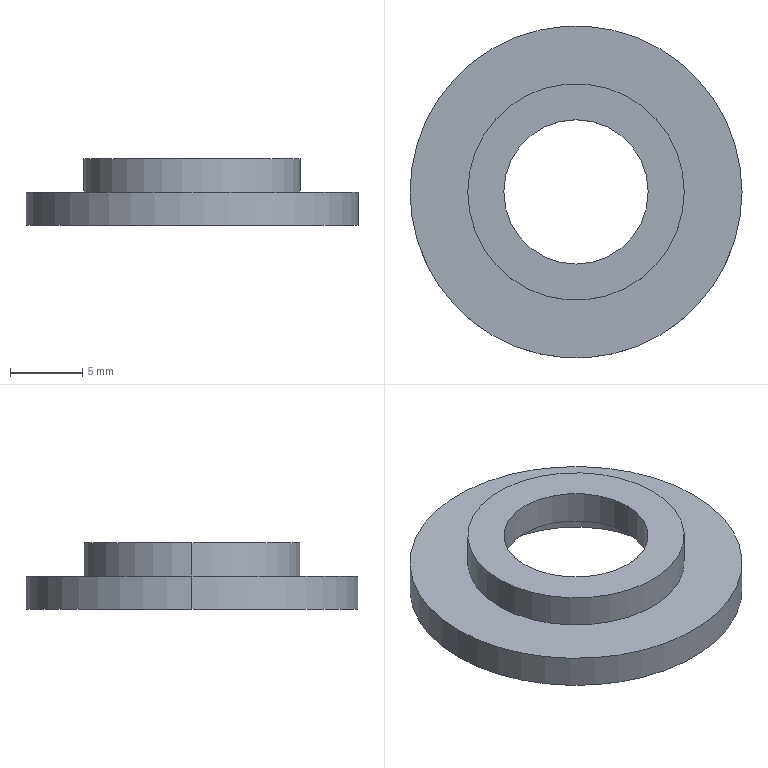Part | SolidWorks | features Extrusion 1, ICE 1 | 2 solids | 12 faces | box 23 x 23 x 4.6 mm | volume 774.952 mm3 | cylinder 8 | plane 4 | commonest cylinder face diameters 15 x4 10 x2 23 x2
STEP:
#1=CARTESIAN_POINT('',(-7.5,0.,2.3));
#2=VERTEX_POINT('',#1);
#3=CARTESIAN_POINT('',(7.5,0.,2.3));
#4=VERTEX_POINT('',#3);
#5=CARTESIAN_POINT('',(0.,0.,2.3));
#6=DIRECTION('',(0.,0.,1.));
#7=DIRECTION('',(1.,0.,0.));
#8=AXIS2_PLACEMENT_3D('',#5,#6,#7);
#9=CIRCLE('',#8,7.5);
#10=EDGE_CURVE('',#2,#4,#9,.T.);
#11=ORIENTED_EDGE('',*,*,#10,.T.);
#12=CARTESIAN_POINT('',(7.5,0.,0.));
#13=VERTEX_POINT('',#12);
#14=CARTESIAN_POINT('',(7.5,0.,2.3));
#15=DIRECTION('',(0.,0.,-1.));
#16=VECTOR('',#15,1000.);
#17=LINE('',#14,#16);
#18=EDGE_CURVE('',#4,#13,#17,.T.);
#19=ORIENTED_EDGE('',*,*,#18,.T.);
#20=CARTESIAN_POINT('',(-7.5,0.,0.));
#21=VERTEX_POINT('',#20);
#22=CARTESIAN_POINT('',(0.,0.,0.));
#23=DIRECTION('',(0.,0.,1.));
#24=DIRECTION('',(1.,0.,0.));
#25=AXIS2_PLACEMENT_3D('',#22,#23,#24);
#26=CIRCLE('',#25,7.5);
#27=EDGE_CURVE('',#21,#13,#26,.T.);
#28=ORIENTED_EDGE('',*,*,#27,.F.);
#29=CARTESIAN_POINT('',(-7.5,0.,2.3));
#30=DIRECTION('',(0.,0.,-1.));
#31=VECTOR('',#30,1000.);
#32=LINE('',#29,#31);
#33=EDGE_CURVE('',#2,#21,#32,.T.);
#34=ORIENTED_EDGE('',*,*,#33,.F.);
#35=EDGE_LOOP('',(#11,#19,#28,#34));
#36=FACE_OUTER_BOUND('',#35,.T.);
#37=CARTESIAN_POINT('',(0.,0.,2.3));
#38=DIRECTION('',(0.,0.,-1.));
#39=DIRECTION('',(-1.,0.,0.));
#40=AXIS2_PLACEMENT_3D('',#37,#38,#39);
#41=CYLINDRICAL_SURFACE('',#40,7.5);
#42=ADVANCED_FACE('',(#36),#41,.F.);
#43=CARTESIAN_POINT('',(11.5,0.,2.3));
#44=VERTEX_POINT('',#43);
#45=CARTESIAN_POINT('',(-11.5,0.,2.3));
#46=VERTEX_POINT('',#45);
#47=CARTESIAN_POINT('',(0.,0.,2.3));
#48=DIRECTION('',(0.,0.,1.));
#49=DIRECTION('',(1.,0.,0.));
#50=AXIS2_PLACEMENT_3D('',#47,#48,#49);
#51=CIRCLE('',#50,11.5);
#52=EDGE_CURVE('',#44,#46,#51,.T.);
#53=ORIENTED_EDGE('',*,*,#52,.F.);
#54=CARTESIAN_POINT('',(11.5,0.,0.));
#55=VERTEX_POINT('',#54);
#56=CARTESIAN_POINT('',(11.5,0.,2.3));
#57=DIRECTION('',(0.,0.,-1.));
#58=VECTOR('',#57,1000.);
#59=LINE('',#56,#58);
#60=EDGE_CURVE('',#44,#55,#59,.T.);
#61=ORIENTED_EDGE('',*,*,#60,.T.);
#62=CARTESIAN_POINT('',(-11.5,0.,0.));
#63=VERTEX_POINT('',#62);
#64=CARTESIAN_POINT('',(0.,0.,0.));
#65=DIRECTION('',(0.,0.,1.));
#66=DIRECTION('',(1.,0.,0.));
#67=AXIS2_PLACEMENT_3D('',#64,#65,#66);
#68=CIRCLE('',#67,11.5);
#69=EDGE_CURVE('',#55,#63,#68,.T.);
#70=ORIENTED_EDGE('',*,*,#69,.T.);
#71=CARTESIAN_POINT('',(-11.5,0.,2.3));
#72=DIRECTION('',(0.,0.,-1.));
#73=VECTOR('',#72,1000.);
#74=LINE('',#71,#73);
#75=EDGE_CURVE('',#46,#63,#74,.T.);
#76=ORIENTED_EDGE('',*,*,#75,.F.);
#77=EDGE_LOOP('',(#53,#61,#70,#76));
#78=FACE_OUTER_BOUND('',#77,.T.);
#79=CARTESIAN_POINT('',(0.,0.,2.3));
#80=DIRECTION('',(0.,0.,-1.));
#81=DIRECTION('',(-1.,0.,0.));
#82=AXIS2_PLACEMENT_3D('',#79,#80,#81);
#83=CYLINDRICAL_SURFACE('',#82,11.5);
#84=ADVANCED_FACE('',(#78),#83,.T.);
#85=CARTESIAN_POINT('',(0.,0.,2.3));
#86=DIRECTION('',(0.,0.,1.));
#87=DIRECTION('',(1.,0.,0.));
#88=AXIS2_PLACEMENT_3D('',#85,#86,#87);
#89=CIRCLE('',#88,11.5);
#90=EDGE_CURVE('',#46,#44,#89,.T.);
#91=ORIENTED_EDGE('',*,*,#90,.T.);
#92=ORIENTED_EDGE('',*,*,#52,.T.);
#93=EDGE_LOOP('',(#91,#92));
#94=FACE_OUTER_BOUND('',#93,.T.);
#95=ORIENTED_EDGE('',*,*,#10,.F.);
#96=CARTESIAN_POINT('',(0.,0.,2.3));
#97=DIRECTION('',(0.,0.,1.));
#98=DIRECTION('',(1.,0.,0.));
#99=AXIS2_PLACEMENT_3D('',#96,#97,#98);
#100=CIRCLE('',#99,7.5);
#101=EDGE_CURVE('',#4,#2,#100,.T.);
#102=ORIENTED_EDGE('',*,*,#101,.F.);
#103=EDGE_LOOP('',(#95,#102));
#104=FACE_BOUND('',#103,.T.);
#105=CARTESIAN_POINT('',(0.,0.,2.3));
#106=DIRECTION('',(0.,0.,1.));
#107=DIRECTION('',(1.,0.,0.));
#108=AXIS2_PLACEMENT_3D('',#105,#106,#107);
#109=PLANE('',#108);
#110=ADVANCED_FACE('',(#94,#104),#109,.T.);
#111=CARTESIAN_POINT('',(0.,0.,0.));
#112=DIRECTION('',(0.,0.,1.));
#113=DIRECTION('',(1.,0.,0.));
#114=AXIS2_PLACEMENT_3D('',#111,#112,#113);
#115=CIRCLE('',#114,11.5);
#116=EDGE_CURVE('',#63,#55,#115,.T.);
#117=ORIENTED_EDGE('',*,*,#116,.F.);
#118=ORIENTED_EDGE('',*,*,#69,.F.);
#119=EDGE_LOOP('',(#117,#118));
#120=FACE_OUTER_BOUND('',#119,.T.);
#121=ORIENTED_EDGE('',*,*,#27,.T.);
#122=CARTESIAN_POINT('',(0.,0.,0.));
#123=DIRECTION('',(0.,0.,1.));
#124=DIRECTION('',(1.,0.,0.));
#125=AXIS2_PLACEMENT_3D('',#122,#123,#124);
#126=CIRCLE('',#125,7.5);
#127=EDGE_CURVE('',#13,#21,#126,.T.);
#128=ORIENTED_EDGE('',*,*,#127,.T.);
#129=EDGE_LOOP('',(#121,#128));
#130=FACE_BOUND('',#129,.T.);
#131=CARTESIAN_POINT('',(0.,0.,0.));
#132=DIRECTION('',(0.,0.,1.));
#133=DIRECTION('',(1.,0.,0.));
#134=AXIS2_PLACEMENT_3D('',#131,#132,#133);
#135=PLANE('',#134);
#136=ADVANCED_FACE('',(#120,#130),#135,.F.);
#137=ORIENTED_EDGE('',*,*,#60,.F.);
#138=ORIENTED_EDGE('',*,*,#90,.F.);
#139=ORIENTED_EDGE('',*,*,#75,.T.);
#140=ORIENTED_EDGE('',*,*,#116,.T.);
#141=EDGE_LOOP('',(#137,#138,#139,#140));
#142=FACE_OUTER_BOUND('',#141,.T.);
#143=CARTESIAN_POINT('',(0.,0.,2.3));
#144=DIRECTION('',(0.,0.,-1.));
#145=DIRECTION('',(-1.,0.,0.));
#146=AXIS2_PLACEMENT_3D('',#143,#144,#145);
#147=CYLINDRICAL_SURFACE('',#146,11.5);
#148=ADVANCED_FACE('',(#142),#147,.T.);
#149=ORIENTED_EDGE('',*,*,#18,.F.);
#150=ORIENTED_EDGE('',*,*,#101,.T.);
#151=ORIENTED_EDGE('',*,*,#33,.T.);
#152=ORIENTED_EDGE('',*,*,#127,.F.);
#153=EDGE_LOOP('',(#149,#150,#151,#152));
#154=FACE_OUTER_BOUND('',#153,.T.);
#155=CARTESIAN_POINT('',(0.,0.,2.3));
#156=DIRECTION('',(0.,0.,-1.));
#157=DIRECTION('',(-1.,0.,0.));
#158=AXIS2_PLACEMENT_3D('',#155,#156,#157);
#159=CYLINDRICAL_SURFACE('',#158,7.5);
#160=ADVANCED_FACE('',(#154),#159,.F.);
#161=CLOSED_SHELL('',(#42,#84,#110,#136,#148,#160));
#162=MANIFOLD_SOLID_BREP('',#161);
#163=CARTESIAN_POINT('',(-5.,0.,4.6));
#164=VERTEX_POINT('',#163);
#165=CARTESIAN_POINT('',(5.,0.,4.6));
#166=VERTEX_POINT('',#165);
#167=CARTESIAN_POINT('',(0.,0.,4.6));
#168=DIRECTION('',(0.,0.,1.));
#169=DIRECTION('',(1.,0.,0.));
#170=AXIS2_PLACEMENT_3D('',#167,#168,#169);
#171=CIRCLE('',#170,5.);
#172=EDGE_CURVE('',#164,#166,#171,.T.);
#173=ORIENTED_EDGE('',*,*,#172,.T.);
#174=CARTESIAN_POINT('',(5.,0.,2.3));
#175=VERTEX_POINT('',#174);
#176=CARTESIAN_POINT('',(5.,0.,4.6));
#177=DIRECTION('',(0.,0.,-1.));
#178=VECTOR('',#177,1000.);
#179=LINE('',#176,#178);
#180=EDGE_CURVE('',#166,#175,#179,.T.);
#181=ORIENTED_EDGE('',*,*,#180,.T.);
#182=CARTESIAN_POINT('',(-5.,0.,2.3));
#183=VERTEX_POINT('',#182);
#184=CARTESIAN_POINT('',(0.,0.,2.3));
#185=DIRECTION('',(0.,0.,1.));
#186=DIRECTION('',(1.,0.,0.));
#187=AXIS2_PLACEMENT_3D('',#184,#185,#186);
#188=CIRCLE('',#187,5.);
#189=EDGE_CURVE('',#183,#175,#188,.T.);
#190=ORIENTED_EDGE('',*,*,#189,.F.);
#191=CARTESIAN_POINT('',(-5.,0.,4.6));
#192=DIRECTION('',(0.,0.,-1.));
#193=VECTOR('',#192,1000.);
#194=LINE('',#191,#193);
#195=EDGE_CURVE('',#164,#183,#194,.T.);
#196=ORIENTED_EDGE('',*,*,#195,.F.);
#197=EDGE_LOOP('',(#173,#181,#190,#196));
#198=FACE_OUTER_BOUND('',#197,.T.);
#199=CARTESIAN_POINT('',(0.,0.,4.6));
#200=DIRECTION('',(0.,0.,-1.));
#201=DIRECTION('',(-1.,0.,0.));
#202=AXIS2_PLACEMENT_3D('',#199,#200,#201);
#203=CYLINDRICAL_SURFACE('',#202,5.);
#204=ADVANCED_FACE('',(#198),#203,.F.);
#205=CARTESIAN_POINT('',(7.5,0.,4.6));
#206=VERTEX_POINT('',#205);
#207=CARTESIAN_POINT('',(-7.5,0.,4.6));
#208=VERTEX_POINT('',#207);
#209=CARTESIAN_POINT('',(0.,0.,4.6));
#210=DIRECTION('',(0.,0.,1.));
#211=DIRECTION('',(1.,0.,0.));
#212=AXIS2_PLACEMENT_3D('',#209,#210,#211);
#213=CIRCLE('',#212,7.5);
#214=EDGE_CURVE('',#206,#208,#213,.T.);
#215=ORIENTED_EDGE('',*,*,#214,.F.);
#216=CARTESIAN_POINT('',(7.5,0.,2.3));
#217=VERTEX_POINT('',#216);
#218=CARTESIAN_POINT('',(7.5,0.,4.6));
#219=DIRECTION('',(0.,0.,-1.));
#220=VECTOR('',#219,1000.);
#221=LINE('',#218,#220);
#222=EDGE_CURVE('',#206,#217,#221,.T.);
#223=ORIENTED_EDGE('',*,*,#222,.T.);
#224=CARTESIAN_POINT('',(-7.5,0.,2.3));
#225=VERTEX_POINT('',#224);
#226=CARTESIAN_POINT('',(0.,0.,2.3));
#227=DIRECTION('',(0.,0.,1.));
#228=DIRECTION('',(1.,0.,0.));
#229=AXIS2_PLACEMENT_3D('',#226,#227,#228);
#230=CIRCLE('',#229,7.5);
#231=EDGE_CURVE('',#217,#225,#230,.T.);
#232=ORIENTED_EDGE('',*,*,#231,.T.);
#233=CARTESIAN_POINT('',(-7.5,0.,4.6));
#234=DIRECTION('',(0.,0.,-1.));
#235=VECTOR('',#234,1000.);
#236=LINE('',#233,#235);
#237=EDGE_CURVE('',#208,#225,#236,.T.);
#238=ORIENTED_EDGE('',*,*,#237,.F.);
#239=EDGE_LOOP('',(#215,#223,#232,#238));
#240=FACE_OUTER_BOUND('',#239,.T.);
#241=CARTESIAN_POINT('',(0.,0.,4.6));
#242=DIRECTION('',(0.,0.,-1.));
#243=DIRECTION('',(-1.,0.,0.));
#244=AXIS2_PLACEMENT_3D('',#241,#242,#243);
#245=CYLINDRICAL_SURFACE('',#244,7.5);
#246=ADVANCED_FACE('',(#240),#245,.T.);
#247=CARTESIAN_POINT('',(0.,0.,4.6));
#248=DIRECTION('',(0.,0.,1.));
#249=DIRECTION('',(1.,0.,0.));
#250=AXIS2_PLACEMENT_3D('',#247,#248,#249);
#251=CIRCLE('',#250,7.5);
#252=EDGE_CURVE('',#208,#206,#251,.T.);
#253=ORIENTED_EDGE('',*,*,#252,.T.);
#254=ORIENTED_EDGE('',*,*,#214,.T.);
#255=EDGE_LOOP('',(#253,#254));
#256=FACE_OUTER_BOUND('',#255,.T.);
#257=ORIENTED_EDGE('',*,*,#172,.F.);
#258=CARTESIAN_POINT('',(0.,0.,4.6));
#259=DIRECTION('',(0.,0.,1.));
#260=DIRECTION('',(1.,0.,0.));
#261=AXIS2_PLACEMENT_3D('',#258,#259,#260);
#262=CIRCLE('',#261,5.);
#263=EDGE_CURVE('',#166,#164,#262,.T.);
#264=ORIENTED_EDGE('',*,*,#263,.F.);
#265=EDGE_LOOP('',(#257,#264));
#266=FACE_BOUND('',#265,.T.);
#267=CARTESIAN_POINT('',(0.,0.,4.6));
#268=DIRECTION('',(0.,0.,1.));
#269=DIRECTION('',(1.,0.,0.));
#270=AXIS2_PLACEMENT_3D('',#267,#268,#269);
#271=PLANE('',#270);
#272=ADVANCED_FACE('',(#256,#266),#271,.T.);
#273=CARTESIAN_POINT('',(0.,0.,2.3));
#274=DIRECTION('',(0.,0.,1.));
#275=DIRECTION('',(1.,0.,0.));
#276=AXIS2_PLACEMENT_3D('',#273,#274,#275);
#277=CIRCLE('',#276,7.5);
#278=EDGE_CURVE('',#225,#217,#277,.T.);
#279=ORIENTED_EDGE('',*,*,#278,.F.);
#280=ORIENTED_EDGE('',*,*,#231,.F.);
#281=EDGE_LOOP('',(#279,#280));
#282=FACE_OUTER_BOUND('',#281,.T.);
#283=ORIENTED_EDGE('',*,*,#189,.T.);
#284=CARTESIAN_POINT('',(0.,0.,2.3));
#285=DIRECTION('',(0.,0.,1.));
#286=DIRECTION('',(1.,0.,0.));
#287=AXIS2_PLACEMENT_3D('',#284,#285,#286);
#288=CIRCLE('',#287,5.);
#289=EDGE_CURVE('',#175,#183,#288,.T.);
#290=ORIENTED_EDGE('',*,*,#289,.T.);
#291=EDGE_LOOP('',(#283,#290));
#292=FACE_BOUND('',#291,.T.);
#293=CARTESIAN_POINT('',(0.,0.,2.3));
#294=DIRECTION('',(0.,0.,1.));
#295=DIRECTION('',(1.,0.,0.));
#296=AXIS2_PLACEMENT_3D('',#293,#294,#295);
#297=PLANE('',#296);
#298=ADVANCED_FACE('',(#282,#292),#297,.F.);
#299=ORIENTED_EDGE('',*,*,#222,.F.);
#300=ORIENTED_EDGE('',*,*,#252,.F.);
#301=ORIENTED_EDGE('',*,*,#237,.T.);
#302=ORIENTED_EDGE('',*,*,#278,.T.);
#303=EDGE_LOOP('',(#299,#300,#301,#302));
#304=FACE_OUTER_BOUND('',#303,.T.);
#305=CARTESIAN_POINT('',(0.,0.,4.6));
#306=DIRECTION('',(0.,0.,-1.));
#307=DIRECTION('',(-1.,0.,0.));
#308=AXIS2_PLACEMENT_3D('',#305,#306,#307);
#309=CYLINDRICAL_SURFACE('',#308,7.5);
#310=ADVANCED_FACE('',(#304),#309,.T.);
#311=ORIENTED_EDGE('',*,*,#180,.F.);
#312=ORIENTED_EDGE('',*,*,#263,.T.);
#313=ORIENTED_EDGE('',*,*,#195,.T.);
#314=ORIENTED_EDGE('',*,*,#289,.F.);
#315=EDGE_LOOP('',(#311,#312,#313,#314));
#316=FACE_OUTER_BOUND('',#315,.T.);
#317=CARTESIAN_POINT('',(0.,0.,4.6));
#318=DIRECTION('',(0.,0.,-1.));
#319=DIRECTION('',(-1.,0.,0.));
#320=AXIS2_PLACEMENT_3D('',#317,#318,#319);
#321=CYLINDRICAL_SURFACE('',#320,5.);
#322=ADVANCED_FACE('',(#316),#321,.F.);
#323=CLOSED_SHELL('',(#204,#246,#272,#298,#310,#322));
#324=MANIFOLD_SOLID_BREP('',#323);
#325=CARTESIAN_POINT('',(0.,0.,0.));
#326=DIRECTION('',(0.,0.,1.));
#327=DIRECTION('',(1.,0.,0.));
#328=AXIS2_PLACEMENT_3D('',#325,#326,#327);
#329=(LENGTH_UNIT()NAMED_UNIT(*)SI_UNIT(.MILLI.,.METRE.));
#330=UNCERTAINTY_MEASURE_WITH_UNIT(LENGTH_MEASURE(0.00001),#329,'','');
#331=(NAMED_UNIT(*)PLANE_ANGLE_UNIT()SI_UNIT($,.RADIAN.));
#332=(NAMED_UNIT(*)SI_UNIT($,.STERADIAN.)SOLID_ANGLE_UNIT());
#333=(GEOMETRIC_REPRESENTATION_CONTEXT(3)GLOBAL_UNCERTAINTY_ASSIGNED_CONTEXT((#330))GLOBAL_UNIT_ASSIGNED_CONTEXT((#329,#331,#332))REPRESENTATION_CONTEXT('',''));
#334=ADVANCED_BREP_SHAPE_REPRESENTATION('',(#162,#324,#328),#333);